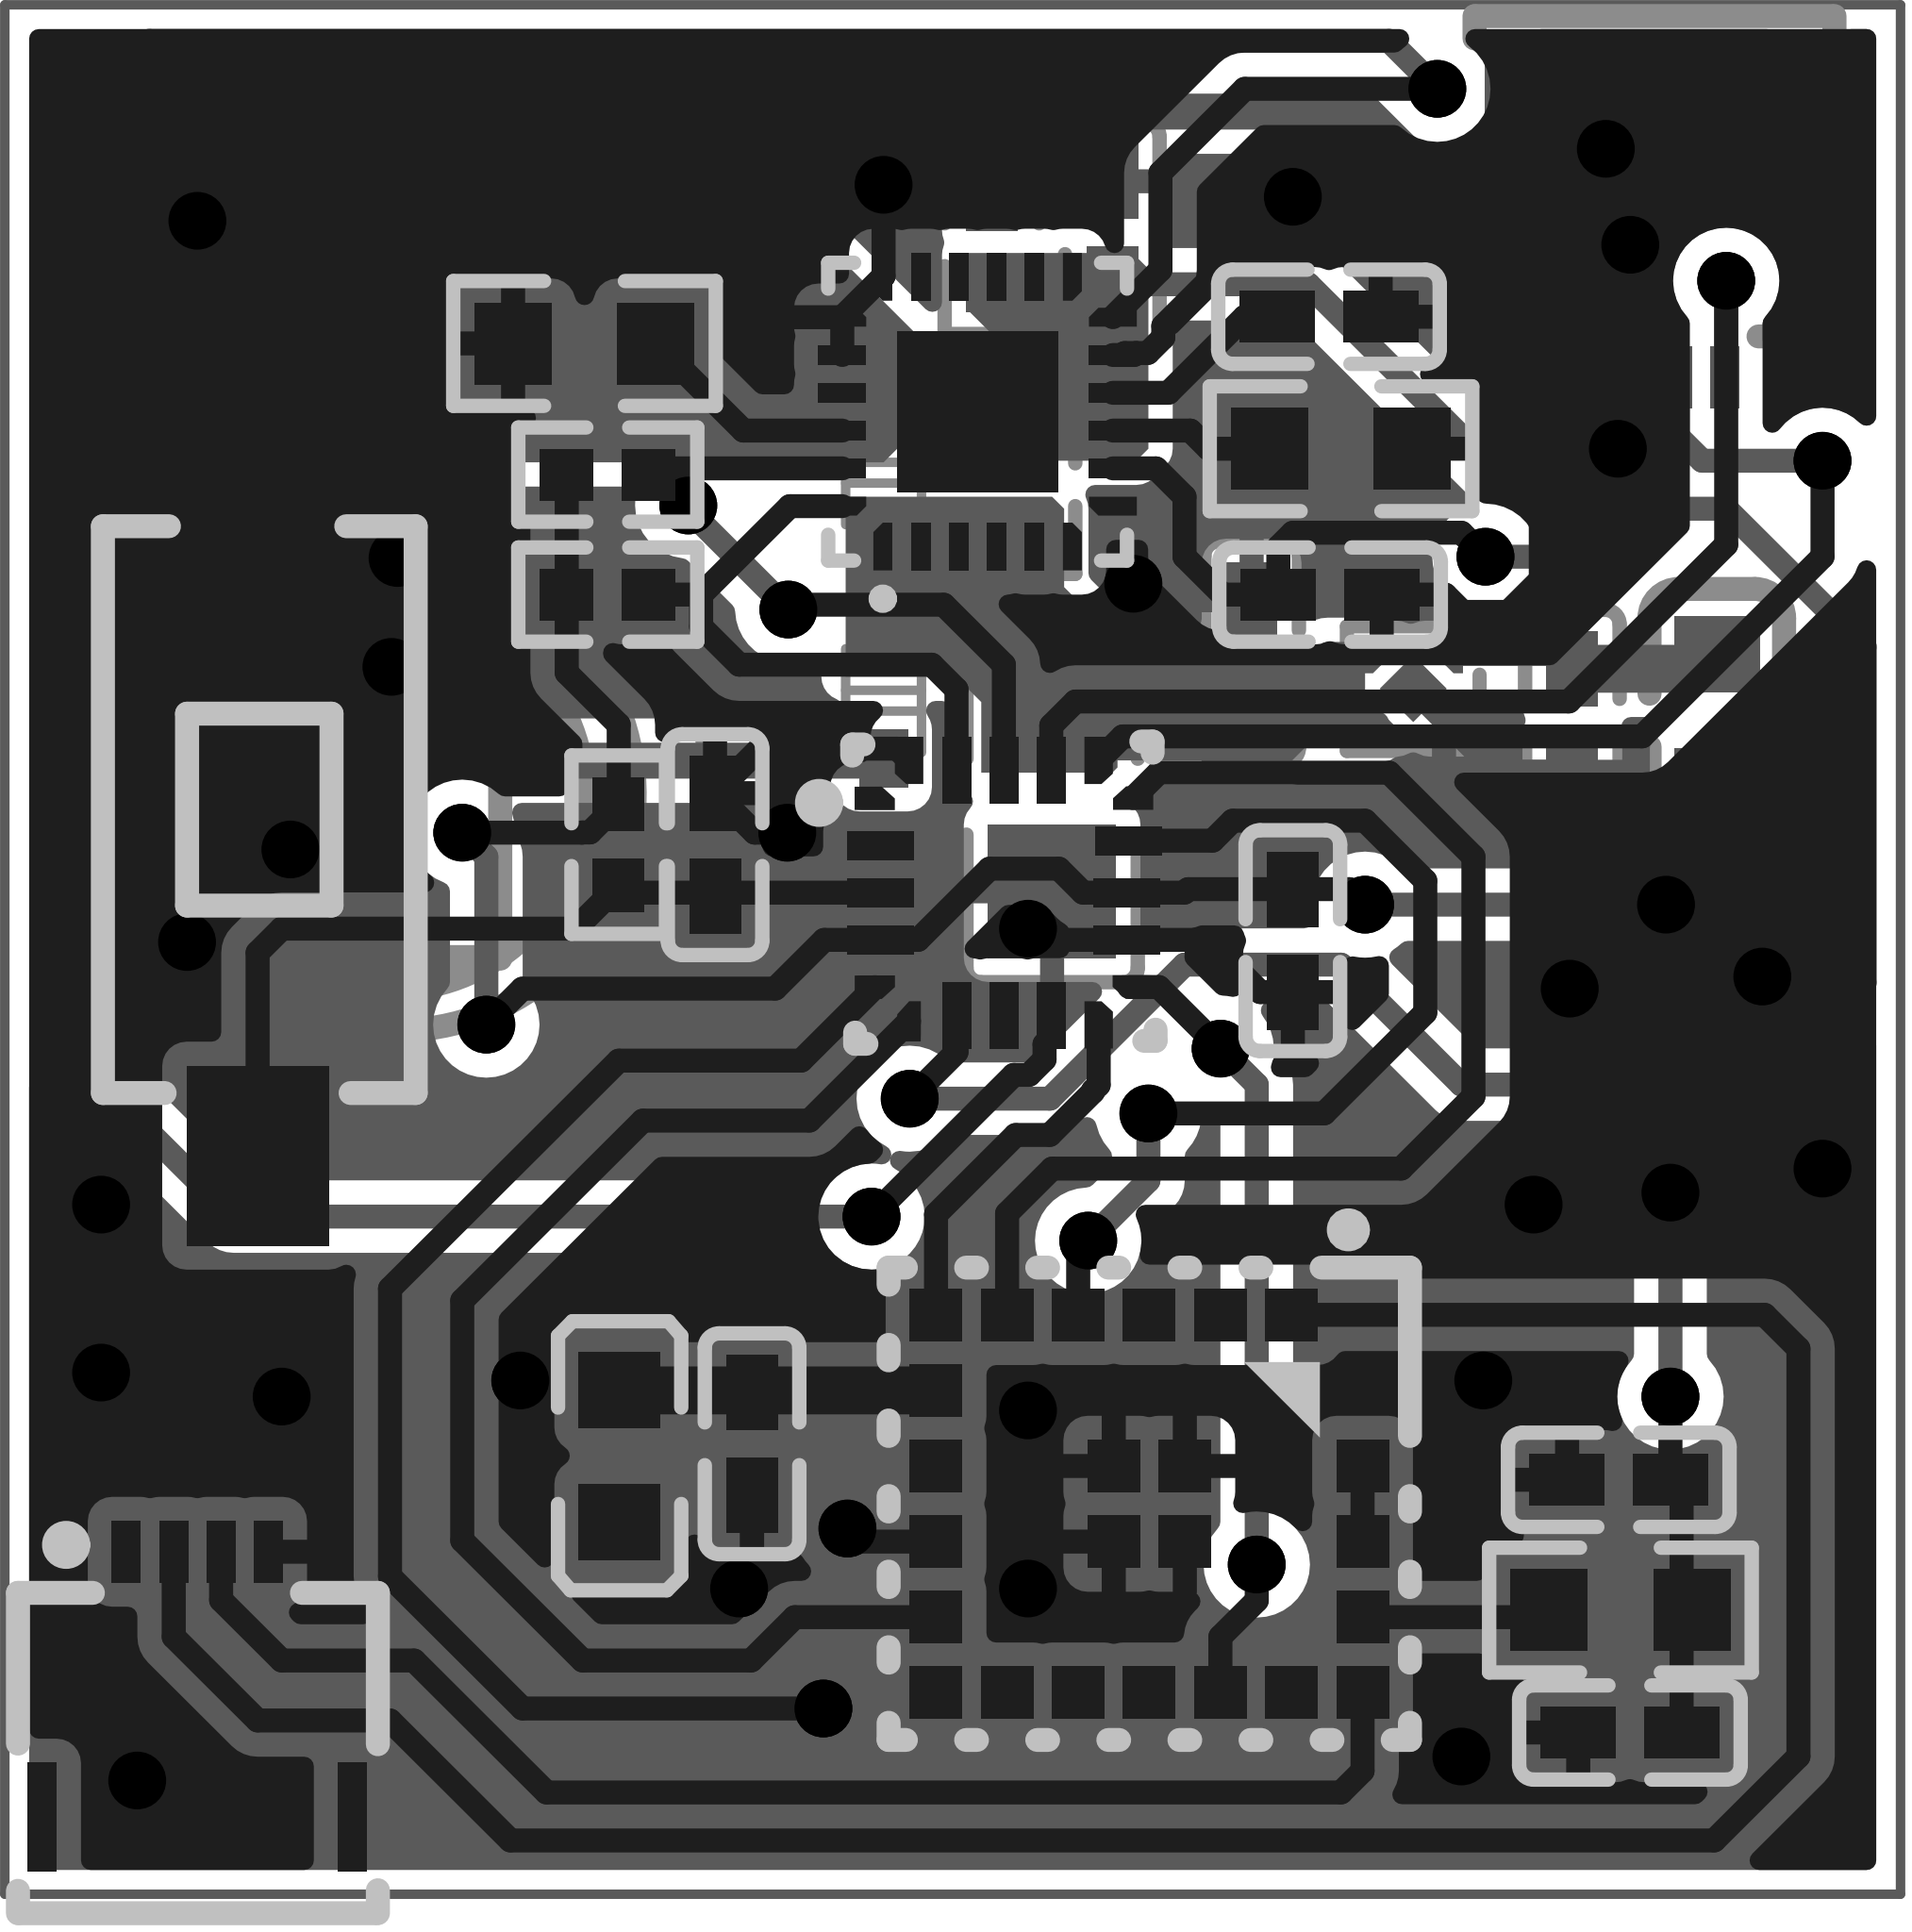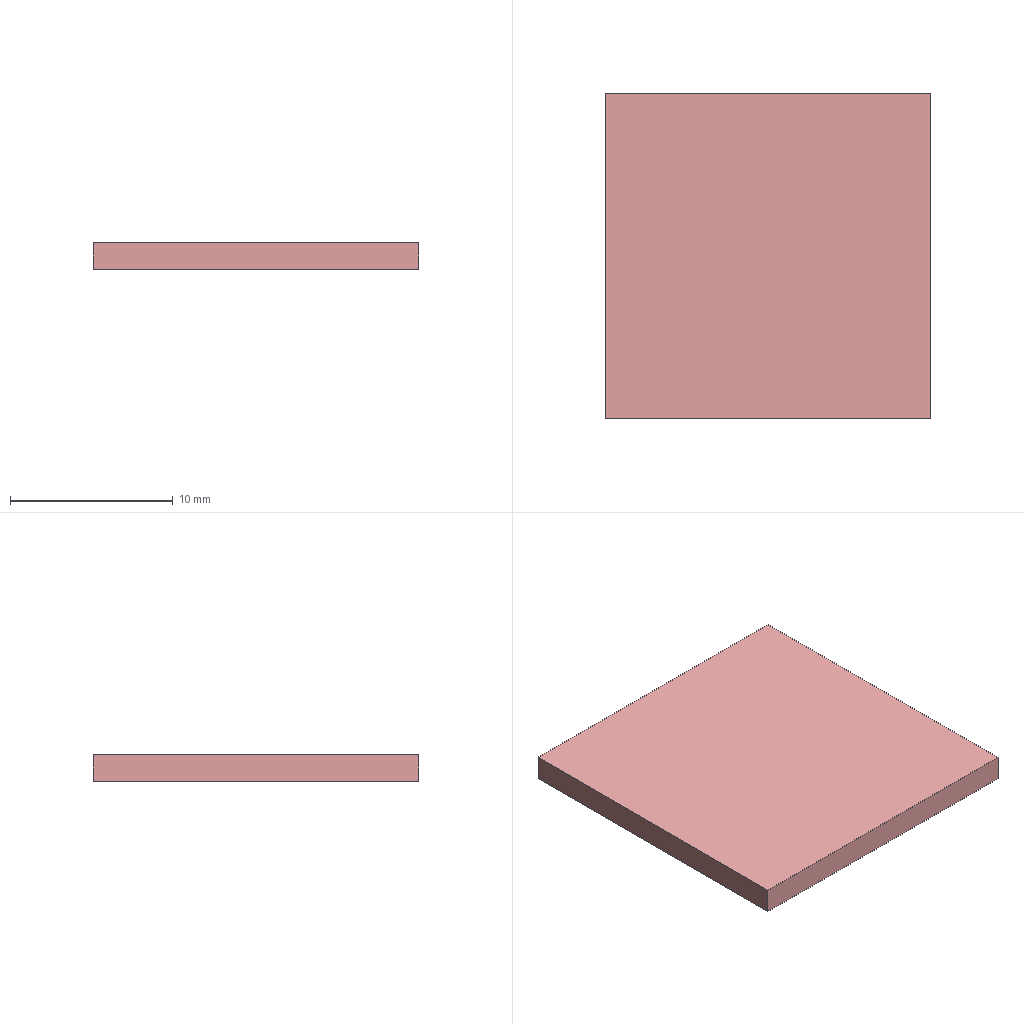Circuit board layout | Altium Designer | box 20 x 20 x 1.6 mm
Layer stack:
# Altium Designer layer stack of  (unit mm; dielectric type: 0 none, 1 core, 2 prepreg, 3 surface material)
index,name,kind,layer,copper_thickness_mm,dielectric_type,dielectric_thickness_mm,dielectric_material,dielectric_constant
0,Top Paste Mask Layer,other,,,,,,
1,Top Silkscreen Layer,other,,,,,,
2,Top Solder Mask Layer,dielectric,,,3,0.01,,3.3
3,Top Layer,copper,Top Layer,0.035,,,,
4,Dielectric1,dielectric,,,3,1.51,FR4,4.5
5,Bottom Layer,copper,Bottom Layer,0.035,,,,
6,Bottom Solder Mask Layer,dielectric,,,3,0.01,,3.3
7,Bottom Silkscreen Layer,other,,,,,,
8,Bottom Paste Mask Layer,other,,,,,,
# drill layer pairs: low layer,high layer
drill_pair,Top Layer,Bottom Layer
Part placement:
Designator,Comment,Layer,Footprint,Center-X(mm),Center-Y(mm),Rotation
C1,1uF,BottomLayer,C0402,95.577,91.45,270
C2,1uF,BottomLayer,C0402,98.961,90.725,90
C4,1uF,TopLayer,C0402,96.012,88.392,90
C5,100nF,TopLayer,C0402,89.916,89.408,270
C6,100nF,TopLayer,C0402,99.568,80.01,0
C7,100nF,TopLayer,C0402,96.404,92.055,180
C8,100nF,TopLayer,C0402,96.393,94.996,0
C9,100nF,TopLayer,C0402,90.306,83.066,90
D1,1N4148G,BottomLayer,SOD-723_L1.0-W0.6-P1.4-RD,91.694,90.932,270
FPC1,HC-FPC-05-10-4RLTAG,BottomLayer,FPC-SMD_4P-P0.50_HCTL_HC-FPC-05-10-4RLTAG,99.822,95.758,180
R6,10kΩ,TopLayer,R0402,88.9,89.408,270
R7,20kΩ,BottomLayer,R0402,93.218,93.218,270
R8,10kΩ,BottomLayer,R0402,92.837,95.758,270
R9,4.7kΩ,TopLayer,R0402,88.784,93.325,0
R10,4.7kΩ,TopLayer,R0402,88.784,92.055,0
STM32L011,STM32L011F4U6TR,TopLayer,QFN-20_L3.0-W3.0-P0.50-BL,92.964,88.9,180
U2,HJ-185IMH,TopLayer,LGA-24_L5.5-W5.0-P0.75-BL-EP,94.497,82.431,180
U3,MS621FE-FL11E,BottomLayer,BAT-SMD_FL11E,86.487,94.996,90
电源模块1,1.8V转压,BottomLayer,ZQFN-4L_L1.0-W1.0-P0.63-BL-EP,97.282,91.06,270
陀螺仪1,ICM-20948,TopLayer,QFN-24_L3.0-W3.0-P0.40-BL-EP,92.686,93.991,0
C10,1uF,BottomLayer,C0402,94.107,95.885,270
C11,100nF,BottomLayer,C0603,100.485,90.725,90
C12,100nF,TopLayer,C0402,99.45,82.685,0
C3,10uF,BottomLayer,C0805,93.472,89.916,90
D2,1N4148G,BottomLayer,SOD-723_L1.0-W0.6-P1.4-RD,91.694,93.345,90
FPC2,HC-FPC-05-10-4RLTAG,TopLayer,FPC-SMD_4P-P0.50_HCTL_HC-FPC-05-10-4RLTAG,84.455,80.518,180
L1,10uH,TopLayer,L0603,88.909,82.939,90
R1,10K,TopLayer,R0603,99.468,81.305,0
R2,10K,TopLayer,R0603,88.539,94.713,0
R3,10K,TopLayer,R0603,96.52,93.599,180
SW1,TS-1101-C-W,TopLayer,SW-SMD_L6.0-W3.3-LS8.0,85.09,89.916,90
Pad and via stacks:
# Altium Designer via and pad stacks of  (unit mm). Each distinct definition once, with the count of objects using it.
# via: kind,start_layer,end_layer,hole_mm,diameter_mm,mode(0 simple;1 top-mid-bottom;2 full stack),diameter_per_layer,count,example_net
# pad: kind,layer,hole_mm,hole_type(0 round;1 square;2 slot),plating,top_size,top_shape(1 round;2 rect;3 octagon;9 rounded rect),mid_size,bottom_size,mode,footprint,size_per_layer,count,example
pad,Bottom Layer,0,0,plated,0.7901x0.54,2,0.7901x0.54,0.7901x0.54,0,C0402,,6,C1.2
pad,Bottom Layer,0,0,plated,0.6096x0.508,2,0.6096x0.508,0.6096x0.508,0,SOD-723_L1.0-W0.6-P1.4-RD,,4,D1.1
pad,Bottom Layer,0,0,plated,0.3x1.15,2,0.3x1.15,0.3x1.15,0,FPC-SMD_4P-P0.50_HCTL_HC-FPC-05-10-4RLTAG,,2,FPC1.6
pad,Bottom Layer,0,0,plated,0.3x0.65,2,0.3x0.65,0.3x0.65,0,FPC-SMD_4P-P0.50_HCTL_HC-FPC-05-10-4RLTAG,,4,FPC1.4
pad,Bottom Layer,0,0,plated,0.5657x0.54,2,0.5657x0.54,0.5657x0.54,0,R0402,,4,R7.2
pad,Bottom Layer,0,0,plated,2.1x0.7,2,2.1x0.7,2.1x0.7,0,BAT-SMD_FL11E,,2,U3.2
pad,Bottom Layer,0,0,plated,0.099x0.099,1,0.099x0.099,0.099x0.099,0,ZQFN-4L_L1.0-W1.0-P0.63-BL-EP,,1,\u7535\u6E90\u6A21\u57571.1
pad,Bottom Layer,0,0,plated,0.1004x0.1004,1,0.1004x0.1004,0.1004x0.1004,0,ZQFN-4L_L1.0-W1.0-P0.63-BL-EP,,2,\u7535\u6E90\u6A21\u57571.3
pad,Bottom Layer,0,0,plated,0.1005x0.1005,1,0.1005x0.1005,0.1005x0.1005,0,ZQFN-4L_L1.0-W1.0-P0.63-BL-EP,,1,\u7535\u6E90\u6A21\u57571.2
pad,Bottom Layer,0,0,plated,0.5x0.5,2,0.5x0.5,0.5x0.5,0,ZQFN-4L_L1.0-W1.0-P0.63-BL-EP,,1,\u7535\u6E90\u6A21\u57571.5
pad,Bottom Layer,0,0,plated,0.8x0.9,2,0.8x0.9,0.8x0.9,0,C0603,,2,C11.2
pad,Bottom Layer,0,0,plated,1.41x1.35,2,1.41x1.35,1.41x1.35,0,C0805,,2,C3.2
pad,Top Layer,0,0,plated,0.7901x0.54,2,0.7901x0.54,0.7901x0.54,0,C0402,,14,C4.2
pad,Top Layer,0,0,plated,0.5657x0.54,2,0.5657x0.54,0.5657x0.54,0,R0402,,6,R6.2
pad,Top Layer,0,0,plated,0.7x0.3,2,0.7x0.3,0.7x0.3,0,QFN-20_L3.0-W3.0-P0.50-BL,,6,STM32L011.4
pad,Top Layer,0,0,plated,0.3x0.7,2,0.3x0.7,0.3x0.7,0,QFN-20_L3.0-W3.0-P0.50-BL,,6,STM32L011.7
pad,Top Layer,0,0,plated,0.1449x0.1449,1,0.1449x0.1449,0.1449x0.1449,0,QFN-20_L3.0-W3.0-P0.50-BL,,3,STM32L011.20
pad,Top Layer,0,0,plated,0.117x0.117,1,0.117x0.117,0.117x0.117,0,QFN-20_L3.0-W3.0-P0.50-BL,,4,STM32L011.5
pad,Top Layer,0,0,plated,0.1169x0.1169,1,0.1169x0.1169,0.1169x0.1169,0,QFN-20_L3.0-W3.0-P0.50-BL,,1,STM32L011.15
pad,Top Layer,0,0,plated,0.55x0.55,2,0.55x0.55,0.55x0.55,0,LGA-24_L5.5-W5.0-P0.75-BL-EP,,24,U2.1
pad,Top Layer,0,0,plated,0.2x0.505,2,0.2x0.505,0.2x0.505,0,QFN-24_L3.0-W3.0-P0.40-BL-EP,,8,\u9640\u87BA\u4EEA1.2
pad,Top Layer,0,0,plated,0.505x0.2,2,0.505x0.2,0.505x0.2,0,QFN-24_L3.0-W3.0-P0.40-BL-EP,,8,\u9640\u87BA\u4EEA1.8
pad,Top Layer,0,0,plated,0.0966x0.0966,1,0.0966x0.0966,0.0966x0.0966,0,QFN-24_L3.0-W3.0-P0.40-BL-EP,,4,\u9640\u87BA\u4EEA1.18
pad,Top Layer,0,0,plated,1.7x1.7,2,1.7x1.7,1.7x1.7,0,QFN-24_L3.0-W3.0-P0.40-BL-EP,,1,\u9640\u87BA\u4EEA1.25
pad,Top Layer,0,0,plated,0.0965x0.0965,1,0.0965x0.0965,0.0965x0.0965,0,QFN-24_L3.0-W3.0-P0.40-BL-EP,,4,\u9640\u87BA\u4EEA1.24
pad,Top Layer,0,0,plated,0.3x1.15,2,0.3x1.15,0.3x1.15,0,FPC-SMD_4P-P0.50_HCTL_HC-FPC-05-10-4RLTAG,,2,FPC2.6
pad,Top Layer,0,0,plated,0.3x0.65,2,0.3x0.65,0.3x0.65,0,FPC-SMD_4P-P0.50_HCTL_HC-FPC-05-10-4RLTAG,,4,FPC2.4
pad,Top Layer,0,0,plated,0.8x0.864,2,0.8x0.864,0.8x0.864,0,L0603,,2,L1.1
pad,Top Layer,0,0,plated,0.8065x0.864,2,0.8065x0.864,0.8065x0.864,0,R0603,,6,R1.2
pad,Top Layer,0,0,plated,1.9x1.5,2,1.9x1.5,1.9x1.5,0,SW-SMD_L6.0-W3.3-LS8.0,,2,SW1.1
via,Top Layer,Bottom Layer,0.3048,0.61,0,,47,SCL
Copper pours:
name,layer,net,type(0 solid;1 hatched;2 none)
Top Layer-GND,Top Layer,GND,0
Bottom Layer-GND,Bottom Layer,GND,0
Design rules, without the lines most boards share:
# Altium Designer design rules of  (exported by Altium Designer, unit mm)
# columns: name | kind | enabled | priority | scope1 | scope2 | descriptor | typed fields (field=value)
otherClearance | 52 | enabled | 1 | All | All | Hole To Hole Clearance (Gap=11.8mil) (All),(All) | gap=0.2997